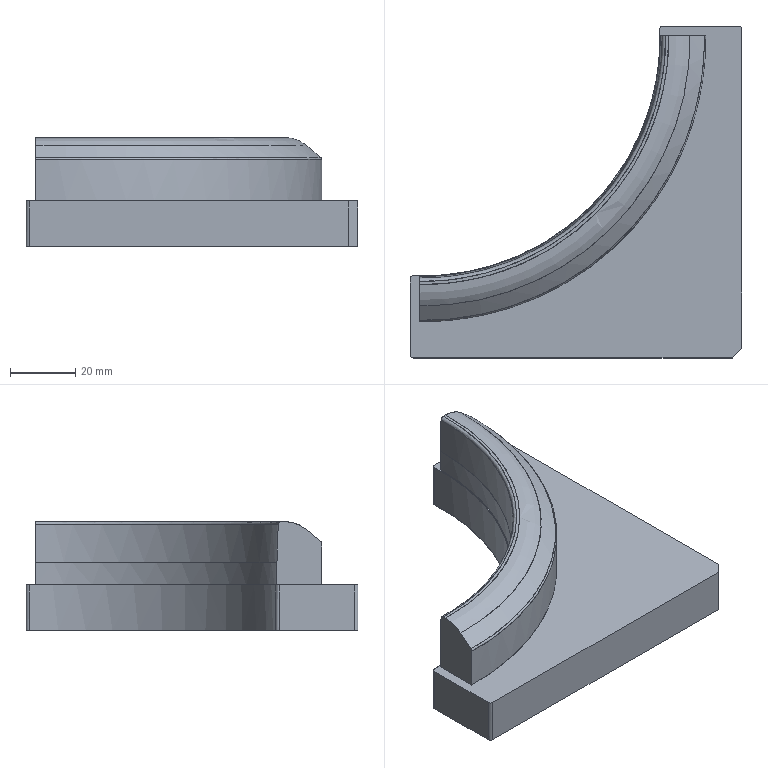NC program | PowerMill | posted with a generic post | part box 102 x 102 x 33.478 mm
Lines 321738 to 321973 of 321973:
N321835 M6
N321836 S15000 M03
N321837 G00 G90 X0.0 Y0.0
N321838 G43 Z10.298 H13
N321839
N321840 G05 P10000 R8
N321841 X-23.9567 Y-47.0628
N321842 Z-19.63
N321843 G01 Z-19.73 F600.0
N321844 X-23.9177 Y-46.8042 F1000.0
N321845 X-23.8509 Y-46.571
N321846 X-23.7561 Y-46.3631
N321847 X-23.6336 Y-46.1806
N321848 X-23.4831 Y-46.0234
N321849 X-23.3076 Y-45.8934
N321850 X-23.1098 Y-45.7923
N321851 X-22.8898 Y-45.72
N321852 X-22.6475 Y-45.6767
N321853 X-22.3829 Y-45.6623
N321854 X-22.1366 Y-45.6761
N321855 X-21.9076 Y-45.7177
N321856 X-21.6961 Y-45.787
N321857 X-21.5019 Y-45.884
N321858 X-21.3251 Y-46.0087
N321859 X-21.1877 Y-46.1399
N321860 X-21.0753 Y-46.2851
N321861 X-20.9879 Y-46.4445
N321862 X-20.9254 Y-46.6181
N321863 X-20.888 Y-46.8057
N321864 X-20.8755 Y-47.0075
N321865 X-20.8879 Y-47.1688
N321866 X-20.9252 Y-47.3319
N321867 X-20.9874 Y-47.4968
N321868 X-21.0745 Y-47.6636
N321869 X-21.1125 Y-47.7167
N321870 X-21.1736 Y-47.7874
N321871 X-21.3646 Y-47.982
N321872 X-21.4947 Y-48.1059
N321873 X-21.5598 Y-48.1547
N321874 X-21.6521 Y-48.2067
N321875 X-21.7715 Y-48.262
N321876 X-21.9181 Y-48.3205
N321877 X-22.0918 Y-48.3823
N321878 X-22.3904 Y-48.4979
N321879 X-22.6703 Y-48.6353
N321880 X-22.9312 Y-48.7945
N321881 X-23.1733 Y-48.9755
N321882 X-23.3965 Y-49.1784
N321883 X-23.582 Y-49.3815
N321884 X-23.738 Y-49.5928
N321885 X-23.8646 Y-49.8123
N321886 X-23.9616 Y-50.04
N321887 X-24.0292 Y-50.2759
N321888 X-24.0673 Y-50.52
N321889 X-20.8718
N321890 G00 Z-16.5904
N321891 G01 X-17.3714 Y-46.3109 F10000.0
N321892 G00 Z-19.63
N321893 G01 Z-19.73 F600.0
N321894 X-16.461 Y-45.6844 F1000.0
N321895 Y-50.52
N321896 G00 Z-16.5904
N321897 G01 X-11.6374 Y-48.8135 F10000.0
N321898 G00 Z-19.63
N321899 G01 Z-19.73 F600.0
N321900 X-13.4913 F1000.0
N321901 G00 Z-16.5904
N321902 G01 X-5.3838 Y-50.52 F10000.0
N321903 G00 Z-19.63
N321904 G01 Z-19.73 F600.0
N321905 X-7.6763 Y-45.6659 F1000.0
N321906 X-9.8914 Y-50.52
N321907 G00 Z-16.5904
N321908 G01 X-6.2959 Y-48.5887 F10000.0
N321909 G00 Z-19.63
N321910 G01 Z-19.73 F600.0
N321911 X-8.9958 F1000.0
N321912 G00 Z-16.5904
N321913 G01 X-1.806 Y-48.8135 F10000.0
N321914 G00 Z-19.63
N321915 G01 Z-19.73 F600.0
N321916 X-3.6598 F1000.0
N321917 G00 Z-16.5904
N321918 G01 X1.5434 Y-46.3109 F10000.0
N321919 G00 Z-19.63
N321920 G01 Z-19.73 F600.0
N321921 X2.4537 Y-45.6844 F1000.0
N321922 Y-50.52
N321923 G00 Z-16.5904
N321924 G01 X7.2773 Y-48.8135 F10000.0
N321925 G00 Z-19.63
N321926 G01 Z-19.73 F600.0
N321927 X5.4234 F1000.0
N321928 G00 Z-16.5904
N321929 G01 X9.3128 Y-48.5001 F10000.0
N321930 G00 Z-19.63
N321931 G01 Z-19.73 F600.0
N321932 X9.3035 Y-48.1354 F1000.0
N321933 X9.3128 Y-47.7695
N321934 X9.3408 Y-47.4329
N321935 X9.3875 Y-47.1256
N321936 X9.4528 Y-46.8476
N321937 X9.5368 Y-46.5988
N321938 X9.6395 Y-46.3793
N321939 X9.7608 Y-46.1891
N321940 X9.9008 Y-46.0281
N321941 X10.0595 Y-45.8964
N321942 X10.2369 Y-45.794
N321943 X10.4329 Y-45.7208
N321944 X10.6476 Y-45.6769
N321945 X10.8809 Y-45.6623
N321946 X11.1143 Y-45.6769
N321947 X11.329 Y-45.7208
N321948 X11.525 Y-45.794
N321949 X11.7023 Y-45.8964
N321950 X11.861 Y-46.0281
N321951 X12.001 Y-46.1891
N321952 X12.1224 Y-46.3793
N321953 X12.2251 Y-46.5988
N321954 X12.3091 Y-46.8476
N321955 X12.3744 Y-47.1256
N321956 X12.4211 Y-47.4329
N321957 X12.4491 Y-47.7695
N321958 X12.4584 Y-48.1354
N321959 X12.4475 Y-48.5218
N321960 X12.4147 Y-48.8757
N321961 X12.3599 Y-49.1972
N321962 X12.2833 Y-49.4862
N321963 X12.1849 Y-49.7427
N321964 X12.0645 Y-49.9667
N321965 X11.9223 Y-50.1582
N321966 X11.7581 Y-50.3173
N321967 X11.6122 Y-50.4195
N321968 X11.4515 Y-50.4989
N321969 X11.276 Y-50.5557
N321970 X11.0859 Y-50.5897
N321971 X10.8809 Y-50.6011
N321972 X10.6476 Y-50.5865
N321973 X10.4329 Y-50.5427
N321974 X10.2369 Y-50.4698
N321975 X10.0595 Y-50.3676
N321976 X9.9008 Y-50.2363
N321977 X9.7608 Y-50.0758
N321978 X9.6395 Y-49.8862
N321979 X9.5368 Y-49.6673
N321980 X9.4528 Y-49.4193
N321981 X9.3875 Y-49.1421
N321982 X9.3408 Y-48.8357
N321983 X9.3128 Y-48.5001
N321984 G00 Z-16.5904
N321985 G01 X15.2291 Y-50.2767 F10000.0
N321986 G00 Z-19.63
N321987 G01 Z-19.73 F600.0
N321988 Y-49.6074 F1000.0
N321989 G00 Z-16.5904
N321990 G01 X18.0985 Y-49.1421 F10000.0
N321991 G00 Z-19.63
N321992 G01 Z-19.73 F600.0
N321993 X18.0518 Y-48.8357 F1000.0
N321994 X18.0238 Y-48.5001
N321995 X18.0145 Y-48.1354
N321996 X18.0238 Y-47.7695
N321997 X18.0518 Y-47.4329
N321998 X18.0985 Y-47.1256
N321999 X18.1638 Y-46.8476
N322000 X18.2478 Y-46.5988
N322001 X18.3505 Y-46.3793
N322002 X18.4718 Y-46.1891
N322003 X18.6119 Y-46.0281
N322004 X18.7705 Y-45.8964
N322005 X18.9479 Y-45.794
N322006 X19.1439 Y-45.7208
N322007 X19.3586 Y-45.6769
N322008 X19.5919 Y-45.6623
N322009 X19.8253 Y-45.6769
N322010 X20.04 Y-45.7208
N322011 X20.236 Y-45.794
N322012 X20.4134 Y-45.8964
N322013 X20.572 Y-46.0281
N322014 X20.712 Y-46.1891
N322015 X20.8334 Y-46.3793
N322016 X20.9361 Y-46.5988
N322017 X21.0201 Y-46.8476
N322018 X21.0854 Y-47.1256
N322019 X21.1321 Y-47.4329
N322020 X21.1601 Y-47.7695
N322021 X21.1694 Y-48.1354
N322022 X21.1585 Y-48.5218
N322023 X21.1257 Y-48.8757
N322024 X21.0709 Y-49.1972
N322025 X20.9944 Y-49.4862
N322026 X20.8959 Y-49.7427
N322027 X20.7755 Y-49.9667
N322028 X20.6333 Y-50.1582
N322029 X20.4691 Y-50.3173
N322030 X20.3232 Y-50.4195
N322031 X20.1625 Y-50.4989
N322032 X19.987 Y-50.5557
N322033 X19.7969 Y-50.5897
N322034 X19.5919 Y-50.6011
N322035 X19.3586 Y-50.5865
N322036 X19.1439 Y-50.5427
N322037 X18.9479 Y-50.4698
N322038 X18.7705 Y-50.3676
N322039 X18.6119 Y-50.2363
N322040 X18.4718 Y-50.0758
N322041 X18.3505 Y-49.8862
N322042 X18.2478 Y-49.6673
N322043 X18.1638 Y-49.4193
N322044 X18.0985 Y-49.1421
N322045 G00 Z-16.5904
N322046 G01 X23.3467 Y-45.747 F10000.0
N322047 G00 Z-19.63
N322048 G01 Z-19.73 F600.0
N322049 X26.4758 F1000.0
N322050 X26.4116 Y-45.9389
N322051 X26.322 Y-46.1534
N322052 X26.207 Y-46.3904
N322053 X26.0667 Y-46.65
N322054 X25.5618 Y-47.5162
N322055 X25.3077 Y-48.0112
N322056 X25.0933 Y-48.5084
N322057 X24.9186 Y-49.0079
N322058 X24.7837 Y-49.5097
N322059 X24.6885 Y-50.0137
N322060 X24.633 Y-50.52
N322061 G00 Z10.298
N322062 G05 P0
N322063 (---------------)
N322064 ( END TOOLPATH : 精公刻字01-刻字-TEXT_D4 )
N322065 (---------------)
N322066
N322067 M05
N322068 G53 Z0.0
N322069 M30
%